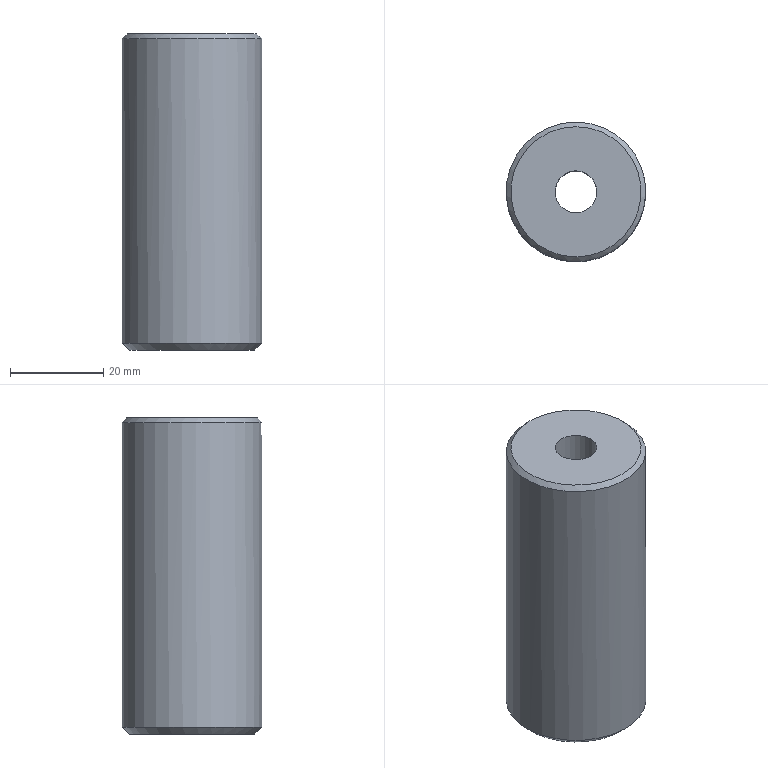Part | STEP file | gslz 2016.10.28-6_id1026_x_t | 1 solid | 8 faces | box 30 x 30 x 67.992 mm | volume 42323 mm3 | plane 3 | cylinder 3 | cone 2 | commonest cylinder face diameters 9 x1 14 x1 30 x1
STEP:
#1=CARTESIAN_POINT('',(50.5,263.,129.992));
#2=VERTEX_POINT('',#1);
#3=CARTESIAN_POINT('',(50.5,249.,129.992));
#4=DIRECTION('',(0.,0.,1.));
#5=DIRECTION('',(0.,1.,0.));
#6=AXIS2_PLACEMENT_3D('',#3,#4,#5);
#7=CIRCLE('',#6,14.);
#8=EDGE_CURVE('',#2,#2,#7,.T.);
#9=ORIENTED_EDGE('',*,*,#8,.T.);
#10=EDGE_LOOP('',(#9));
#11=FACE_BOUND('',#10,.T.);
#12=CARTESIAN_POINT('',(50.5,244.5,129.992));
#13=VERTEX_POINT('',#12);
#14=CARTESIAN_POINT('',(50.5,249.,129.992));
#15=DIRECTION('',(0.,0.,1.));
#16=DIRECTION('',(0.,-1.,0.));
#17=AXIS2_PLACEMENT_3D('',#14,#15,#16);
#18=CIRCLE('',#17,4.5);
#19=EDGE_CURVE('',#13,#13,#18,.T.);
#20=ORIENTED_EDGE('',*,*,#19,.F.);
#21=EDGE_LOOP('',(#20));
#22=FACE_BOUND('',#21,.T.);
#23=CARTESIAN_POINT('',(-19.,155.,129.992));
#24=DIRECTION('',(0.,0.,-1.));
#25=DIRECTION('',(1.,0.,0.));
#26=AXIS2_PLACEMENT_3D('',#23,#24,#25);
#27=PLANE('',#26);
#28=ADVANCED_FACE('',(#11,#22),#27,.F.);
#29=CARTESIAN_POINT('',(50.5,264.,63.5));
#30=VERTEX_POINT('',#29);
#31=CARTESIAN_POINT('',(50.5,249.,63.5));
#32=DIRECTION('',(0.,0.,1.));
#33=DIRECTION('',(0.,1.,0.));
#34=AXIS2_PLACEMENT_3D('',#31,#32,#33);
#35=CIRCLE('',#34,15.);
#36=EDGE_CURVE('',#30,#30,#35,.T.);
#37=ORIENTED_EDGE('',*,*,#36,.T.);
#38=EDGE_LOOP('',(#37));
#39=FACE_BOUND('',#38,.T.);
#40=CARTESIAN_POINT('',(50.5,264.,128.992));
#41=VERTEX_POINT('',#40);
#42=CARTESIAN_POINT('',(50.5,249.,128.992));
#43=DIRECTION('',(0.,0.,-1.));
#44=DIRECTION('',(0.,1.,0.));
#45=AXIS2_PLACEMENT_3D('',#42,#43,#44);
#46=CIRCLE('',#45,15.);
#47=EDGE_CURVE('',#41,#41,#46,.T.);
#48=ORIENTED_EDGE('',*,*,#47,.T.);
#49=EDGE_LOOP('',(#48));
#50=FACE_BOUND('',#49,.T.);
#51=CARTESIAN_POINT('',(50.5,249.,86.5));
#52=DIRECTION('',(0.,0.,-1.));
#53=DIRECTION('',(0.,1.,0.));
#54=AXIS2_PLACEMENT_3D('',#51,#52,#53);
#55=CYLINDRICAL_SURFACE('',#54,15.);
#56=ADVANCED_FACE('',(#39,#50),#55,.T.);
#57=CARTESIAN_POINT('',(50.5,242.,62.));
#58=VERTEX_POINT('',#57);
#59=CARTESIAN_POINT('',(50.5,249.,62.));
#60=DIRECTION('',(0.,0.,-1.));
#61=DIRECTION('',(0.,-1.,0.));
#62=AXIS2_PLACEMENT_3D('',#59,#60,#61);
#63=CIRCLE('',#62,7.);
#64=EDGE_CURVE('',#58,#58,#63,.T.);
#65=ORIENTED_EDGE('',*,*,#64,.F.);
#66=EDGE_LOOP('',(#65));
#67=FACE_BOUND('',#66,.T.);
#68=CARTESIAN_POINT('',(64.,249.,62.));
#69=VERTEX_POINT('',#68);
#70=CARTESIAN_POINT('',(50.5,249.,62.));
#71=DIRECTION('',(0.,0.,-1.));
#72=DIRECTION('',(1.,0.,0.));
#73=AXIS2_PLACEMENT_3D('',#70,#71,#72);
#74=CIRCLE('',#73,13.5);
#75=EDGE_CURVE('',#69,#69,#74,.T.);
#76=ORIENTED_EDGE('',*,*,#75,.T.);
#77=EDGE_LOOP('',(#76));
#78=FACE_BOUND('',#77,.T.);
#79=CARTESIAN_POINT('',(20.5,204.,62.));
#80=DIRECTION('',(0.,0.,1.));
#81=DIRECTION('',(-1.,0.,0.));
#82=AXIS2_PLACEMENT_3D('',#79,#80,#81);
#83=PLANE('',#82);
#84=ADVANCED_FACE('',(#67,#78),#83,.F.);
#85=ORIENTED_EDGE('',*,*,#8,.F.);
#86=EDGE_LOOP('',(#85));
#87=FACE_BOUND('',#86,.T.);
#88=ORIENTED_EDGE('',*,*,#47,.F.);
#89=EDGE_LOOP('',(#88));
#90=FACE_BOUND('',#89,.T.);
#91=CARTESIAN_POINT('',(50.5,249.,128.992));
#92=DIRECTION('',(0.,0.,-1.));
#93=DIRECTION('',(0.,1.,0.));
#94=AXIS2_PLACEMENT_3D('',#91,#92,#93);
#95=CONICAL_SURFACE('',#94,15.,45.);
#96=ADVANCED_FACE('',(#87,#90),#95,.T.);
#97=ORIENTED_EDGE('',*,*,#36,.F.);
#98=EDGE_LOOP('',(#97));
#99=FACE_BOUND('',#98,.T.);
#100=ORIENTED_EDGE('',*,*,#75,.F.);
#101=EDGE_LOOP('',(#100));
#102=FACE_BOUND('',#101,.T.);
#103=CARTESIAN_POINT('',(50.5,249.,62.));
#104=DIRECTION('',(0.,0.,1.));
#105=DIRECTION('',(0.,-1.,0.));
#106=AXIS2_PLACEMENT_3D('',#103,#104,#105);
#107=CONICAL_SURFACE('',#106,13.5,45.);
#108=ADVANCED_FACE('',(#99,#102),#107,.T.);
#109=ORIENTED_EDGE('',*,*,#19,.T.);
#110=EDGE_LOOP('',(#109));
#111=FACE_BOUND('',#110,.T.);
#112=CARTESIAN_POINT('',(50.5,244.5,75.992));
#113=VERTEX_POINT('',#112);
#114=CARTESIAN_POINT('',(50.5,249.,75.992));
#115=DIRECTION('',(0.,0.,-1.));
#116=DIRECTION('',(0.,-1.,0.));
#117=AXIS2_PLACEMENT_3D('',#114,#115,#116);
#118=CIRCLE('',#117,4.5);
#119=EDGE_CURVE('',#113,#113,#118,.T.);
#120=ORIENTED_EDGE('',*,*,#119,.T.);
#121=EDGE_LOOP('',(#120));
#122=FACE_BOUND('',#121,.T.);
#123=CARTESIAN_POINT('',(50.5,249.,129.992));
#124=DIRECTION('',(0.,0.,1.));
#125=DIRECTION('',(1.,0.,0.));
#126=AXIS2_PLACEMENT_3D('',#123,#124,#125);
#127=CYLINDRICAL_SURFACE('',#126,4.5);
#128=ADVANCED_FACE('',(#111,#122),#127,.F.);
#129=ORIENTED_EDGE('',*,*,#119,.F.);
#130=EDGE_LOOP('',(#129));
#131=FACE_BOUND('',#130,.T.);
#132=CARTESIAN_POINT('',(50.5,242.,75.992));
#133=VERTEX_POINT('',#132);
#134=CARTESIAN_POINT('',(50.5,249.,75.992));
#135=DIRECTION('',(0.,0.,-1.));
#136=DIRECTION('',(0.,-1.,0.));
#137=AXIS2_PLACEMENT_3D('',#134,#135,#136);
#138=CIRCLE('',#137,7.);
#139=EDGE_CURVE('',#133,#133,#138,.T.);
#140=ORIENTED_EDGE('',*,*,#139,.T.);
#141=EDGE_LOOP('',(#140));
#142=FACE_BOUND('',#141,.T.);
#143=CARTESIAN_POINT('',(50.5,249.,75.992));
#144=DIRECTION('',(0.,0.,1.));
#145=DIRECTION('',(0.,1.,0.));
#146=AXIS2_PLACEMENT_3D('',#143,#144,#145);
#147=PLANE('',#146);
#148=ADVANCED_FACE('',(#131,#142),#147,.F.);
#149=ORIENTED_EDGE('',*,*,#64,.T.);
#150=EDGE_LOOP('',(#149));
#151=FACE_BOUND('',#150,.T.);
#152=ORIENTED_EDGE('',*,*,#139,.F.);
#153=EDGE_LOOP('',(#152));
#154=FACE_BOUND('',#153,.T.);
#155=CARTESIAN_POINT('',(50.5,249.,64.992));
#156=DIRECTION('',(0.,0.,1.));
#157=DIRECTION('',(1.,0.,0.));
#158=AXIS2_PLACEMENT_3D('',#155,#156,#157);
#159=CYLINDRICAL_SURFACE('',#158,7.);
#160=ADVANCED_FACE('',(#151,#154),#159,.F.);
#161=CLOSED_SHELL('',(#28,#56,#84,#96,#108,#128,#148,#160));
#162=MANIFOLD_SOLID_BREP('',#161);
#163=(LENGTH_UNIT()NAMED_UNIT(*)SI_UNIT(.MILLI.,.METRE.));
#164=UNCERTAINTY_MEASURE_WITH_UNIT(LENGTH_MEASURE(0.00002),#163,'','');
#165=(NAMED_UNIT(*)PLANE_ANGLE_UNIT()SI_UNIT($,.RADIAN.));
#166=PLANE_ANGLE_MEASURE_WITH_UNIT(PLANE_ANGLE_MEASURE(0.01745),#165);
#167=DIMENSIONAL_EXPONENTS(0.,0.,0.,0.,0.,0.,0.);
#168=(CONVERSION_BASED_UNIT('DEGREE',#166)NAMED_UNIT(#167)PLANE_ANGLE_UNIT());
#169=(NAMED_UNIT(*)SI_UNIT($,.STERADIAN.)SOLID_ANGLE_UNIT());
#170=(GEOMETRIC_REPRESENTATION_CONTEXT(3)GLOBAL_UNCERTAINTY_ASSIGNED_CONTEXT((#164))GLOBAL_UNIT_ASSIGNED_CONTEXT((#163,#168,#169))REPRESENTATION_CONTEXT('',''));
#171=ADVANCED_BREP_SHAPE_REPRESENTATION('',(#162),#170);